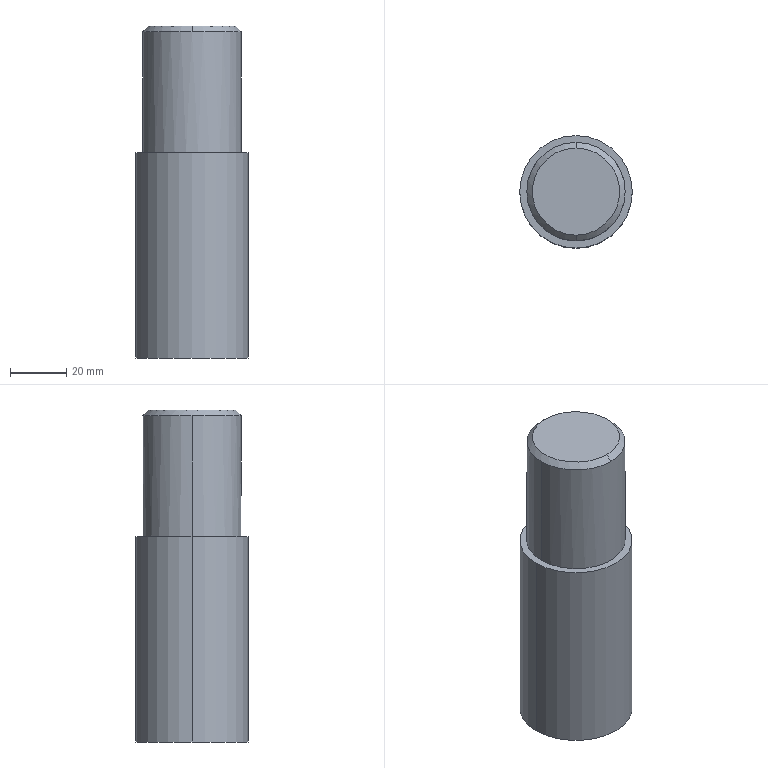Part | STEP file | PISTON XYLANH _S_^80 | 1 solid | 9 faces | box 40 x 40 x 118 mm | volume 134818 mm3 | cylinder 4 | plane 3 | cone 2 | commonest cylinder face diameters 35 x2 40 x2
STEP:
#1=CARTESIAN_POINT('',(0.,0.,0.));
#2=DIRECTION('',(0.,0.,1.));
#3=DIRECTION('',(1.,0.,0.));
#4=AXIS2_PLACEMENT_3D('',#1,#2,#3);
#5=CARTESIAN_POINT('',(20.,0.,0.));
#6=VERTEX_POINT('',#5);
#7=CARTESIAN_POINT('',(-20.,0.,0.));
#8=VERTEX_POINT('',#7);
#9=CARTESIAN_POINT('',(0.,0.,0.));
#10=DIRECTION('',(0.,0.,1.));
#11=DIRECTION('',(1.,0.,0.));
#12=AXIS2_PLACEMENT_3D('',#9,#10,#11);
#13=CIRCLE('',#12,20.);
#14=CARTESIAN_POINT('',(0.,0.,0.));
#15=DIRECTION('',(0.,0.,1.));
#16=DIRECTION('',(1.,0.,0.));
#17=AXIS2_PLACEMENT_3D('',#14,#15,#16);
#18=CYLINDRICAL_SURFACE('',#17,20.);
#19=CARTESIAN_POINT('',(0.,0.));
#20=DIRECTION('',(1.,0.));
#21=VECTOR('',#20,1.);
#22=LINE('',#19,#21);
#23=(GEOMETRIC_REPRESENTATION_CONTEXT(2)PARAMETRIC_REPRESENTATION_CONTEXT()REPRESENTATION_CONTEXT('',''));
#24=DEFINITIONAL_REPRESENTATION('',(#22),#23);
#25=PCURVE('',#18,#24);
#26=CARTESIAN_POINT('',(0.,0.,0.));
#27=DIRECTION('',(0.,0.,-1.));
#28=DIRECTION('',(-1.,0.,0.));
#29=AXIS2_PLACEMENT_3D('',#26,#27,#28);
#30=PLANE('',#29);
#31=CARTESIAN_POINT('',(-20.,0.));
#32=CARTESIAN_POINT('',(-20.,34.641));
#33=CARTESIAN_POINT('',(10.,17.321));
#34=CARTESIAN_POINT('',(40.,0.));
#35=CARTESIAN_POINT('',(10.,-17.321));
#36=CARTESIAN_POINT('',(-20.,-34.641));
#37=CARTESIAN_POINT('',(-20.,0.));
#38=(BOUNDED_CURVE()B_SPLINE_CURVE(2,(#31,#32,#33,#34,#35,#36,#37),.UNSPECIFIED.,.T.,.F.)B_SPLINE_CURVE_WITH_KNOTS((1,2,2,2,2,1),(-2.094,0.,2.094,4.189,6.283,8.378),.UNSPECIFIED.)CURVE()GEOMETRIC_REPRESENTATION_ITEM()RATIONAL_B_SPLINE_CURVE((1.,0.5,1.,0.5,1.,0.5,1.))REPRESENTATION_ITEM(''));
#39=(GEOMETRIC_REPRESENTATION_CONTEXT(2)PARAMETRIC_REPRESENTATION_CONTEXT()REPRESENTATION_CONTEXT('',''));
#40=DEFINITIONAL_REPRESENTATION('',(#38),#39);
#41=PCURVE('',#30,#40);
#42=SURFACE_CURVE('',#13,(#25,#41),.PCURVE_S1.);
#43=EDGE_CURVE('',#6,#8,#42,.T.);
#44=ORIENTED_EDGE('',*,*,#43,.T.);
#45=CARTESIAN_POINT('',(-20.,0.,73.));
#46=VERTEX_POINT('',#45);
#47=CARTESIAN_POINT('',(-20.,0.,0.));
#48=DIRECTION('',(0.,0.,1.));
#49=VECTOR('',#48,1.);
#50=LINE('',#47,#49);
#51=CARTESIAN_POINT('',(3.142,0.));
#52=DIRECTION('',(0.,1.));
#53=VECTOR('',#52,1.);
#54=LINE('',#51,#53);
#55=(GEOMETRIC_REPRESENTATION_CONTEXT(2)PARAMETRIC_REPRESENTATION_CONTEXT()REPRESENTATION_CONTEXT('',''));
#56=DEFINITIONAL_REPRESENTATION('',(#54),#55);
#57=PCURVE('',#18,#56);
#58=CARTESIAN_POINT('',(0.,0.,0.));
#59=DIRECTION('',(0.,0.,1.));
#60=DIRECTION('',(1.,0.,0.));
#61=AXIS2_PLACEMENT_3D('',#58,#59,#60);
#62=CYLINDRICAL_SURFACE('',#61,20.);
#63=CARTESIAN_POINT('',(3.142,0.));
#64=DIRECTION('',(0.,1.));
#65=VECTOR('',#64,1.);
#66=LINE('',#63,#65);
#67=(GEOMETRIC_REPRESENTATION_CONTEXT(2)PARAMETRIC_REPRESENTATION_CONTEXT()REPRESENTATION_CONTEXT('',''));
#68=DEFINITIONAL_REPRESENTATION('',(#66),#67);
#69=PCURVE('',#62,#68);
#70=SURFACE_CURVE('',#50,(#57,#69),.PCURVE_S1.);
#71=EDGE_CURVE('',#8,#46,#70,.T.);
#72=ORIENTED_EDGE('',*,*,#71,.T.);
#73=CARTESIAN_POINT('',(20.,0.,73.));
#74=VERTEX_POINT('',#73);
#75=CARTESIAN_POINT('',(0.,0.,73.));
#76=DIRECTION('',(0.,0.,-1.));
#77=DIRECTION('',(1.,0.,0.));
#78=AXIS2_PLACEMENT_3D('',#75,#76,#77);
#79=CIRCLE('',#78,20.);
#80=CARTESIAN_POINT('',(6.283,73.));
#81=DIRECTION('',(-1.,0.));
#82=VECTOR('',#81,1.);
#83=LINE('',#80,#82);
#84=(GEOMETRIC_REPRESENTATION_CONTEXT(2)PARAMETRIC_REPRESENTATION_CONTEXT()REPRESENTATION_CONTEXT('',''));
#85=DEFINITIONAL_REPRESENTATION('',(#83),#84);
#86=PCURVE('',#18,#85);
#87=CARTESIAN_POINT('',(0.,0.,73.));
#88=DIRECTION('',(0.,0.,-1.));
#89=DIRECTION('',(-1.,0.,0.));
#90=AXIS2_PLACEMENT_3D('',#87,#88,#89);
#91=PLANE('',#90);
#92=CARTESIAN_POINT('',(0.,0.));
#93=DIRECTION('',(-1.,0.));
#94=AXIS2_PLACEMENT_2D('',#92,#93);
#95=CIRCLE('',#94,20.);
#96=(GEOMETRIC_REPRESENTATION_CONTEXT(2)PARAMETRIC_REPRESENTATION_CONTEXT()REPRESENTATION_CONTEXT('',''));
#97=DEFINITIONAL_REPRESENTATION('',(#95),#96);
#98=PCURVE('',#91,#97);
#99=SURFACE_CURVE('',#79,(#86,#98),.PCURVE_S1.);
#100=EDGE_CURVE('',#46,#74,#99,.T.);
#101=ORIENTED_EDGE('',*,*,#100,.T.);
#102=CARTESIAN_POINT('',(20.,0.,0.));
#103=DIRECTION('',(0.,0.,1.));
#104=VECTOR('',#103,1.);
#105=LINE('',#102,#104);
#106=CARTESIAN_POINT('',(0.,0.));
#107=DIRECTION('',(0.,1.));
#108=VECTOR('',#107,1.);
#109=LINE('',#106,#108);
#110=(GEOMETRIC_REPRESENTATION_CONTEXT(2)PARAMETRIC_REPRESENTATION_CONTEXT()REPRESENTATION_CONTEXT('',''));
#111=DEFINITIONAL_REPRESENTATION('',(#109),#110);
#112=PCURVE('',#18,#111);
#113=CARTESIAN_POINT('',(6.283,0.));
#114=DIRECTION('',(0.,1.));
#115=VECTOR('',#114,1.);
#116=LINE('',#113,#115);
#117=(GEOMETRIC_REPRESENTATION_CONTEXT(2)PARAMETRIC_REPRESENTATION_CONTEXT()REPRESENTATION_CONTEXT('',''));
#118=DEFINITIONAL_REPRESENTATION('',(#116),#117);
#119=PCURVE('',#62,#118);
#120=SURFACE_CURVE('',#105,(#112,#119),.PCURVE_S1.);
#121=EDGE_CURVE('',#6,#74,#120,.T.);
#122=ORIENTED_EDGE('',*,*,#121,.F.);
#123=EDGE_LOOP('',(#44,#72,#101,#122));
#124=FACE_BOUND('',#123,.T.);
#125=ADVANCED_FACE('',(#124),#18,.T.);
#126=CARTESIAN_POINT('',(17.5,0.,73.));
#127=VERTEX_POINT('',#126);
#128=CARTESIAN_POINT('',(-17.5,0.,73.));
#129=VERTEX_POINT('',#128);
#130=CARTESIAN_POINT('',(0.,0.,73.));
#131=DIRECTION('',(0.,0.,1.));
#132=DIRECTION('',(1.,0.,0.));
#133=AXIS2_PLACEMENT_3D('',#130,#131,#132);
#134=CIRCLE('',#133,17.5);
#135=CARTESIAN_POINT('',(0.,0.,73.));
#136=DIRECTION('',(0.,0.,1.));
#137=DIRECTION('',(1.,0.,0.));
#138=AXIS2_PLACEMENT_3D('',#135,#136,#137);
#139=CYLINDRICAL_SURFACE('',#138,17.5);
#140=CARTESIAN_POINT('',(0.,0.));
#141=DIRECTION('',(1.,0.));
#142=VECTOR('',#141,1.);
#143=LINE('',#140,#142);
#144=(GEOMETRIC_REPRESENTATION_CONTEXT(2)PARAMETRIC_REPRESENTATION_CONTEXT()REPRESENTATION_CONTEXT('',''));
#145=DEFINITIONAL_REPRESENTATION('',(#143),#144);
#146=PCURVE('',#139,#145);
#147=CARTESIAN_POINT('',(-17.5,0.));
#148=CARTESIAN_POINT('',(-17.5,30.311));
#149=CARTESIAN_POINT('',(8.75,15.155));
#150=CARTESIAN_POINT('',(35.,0.));
#151=CARTESIAN_POINT('',(8.75,-15.155));
#152=CARTESIAN_POINT('',(-17.5,-30.311));
#153=CARTESIAN_POINT('',(-17.5,0.));
#154=(BOUNDED_CURVE()B_SPLINE_CURVE(2,(#147,#148,#149,#150,#151,#152,#153),.UNSPECIFIED.,.T.,.F.)B_SPLINE_CURVE_WITH_KNOTS((1,2,2,2,2,1),(-2.094,0.,2.094,4.189,6.283,8.378),.UNSPECIFIED.)CURVE()GEOMETRIC_REPRESENTATION_ITEM()RATIONAL_B_SPLINE_CURVE((1.,0.5,1.,0.5,1.,0.5,1.))REPRESENTATION_ITEM(''));
#155=(GEOMETRIC_REPRESENTATION_CONTEXT(2)PARAMETRIC_REPRESENTATION_CONTEXT()REPRESENTATION_CONTEXT('',''));
#156=DEFINITIONAL_REPRESENTATION('',(#154),#155);
#157=PCURVE('',#91,#156);
#158=SURFACE_CURVE('',#134,(#146,#157),.PCURVE_S1.);
#159=EDGE_CURVE('',#127,#129,#158,.T.);
#160=ORIENTED_EDGE('',*,*,#159,.T.);
#161=CARTESIAN_POINT('',(-17.5,0.,116.));
#162=VERTEX_POINT('',#161);
#163=CARTESIAN_POINT('',(-17.5,0.,73.));
#164=DIRECTION('',(0.,0.,1.));
#165=VECTOR('',#164,1.);
#166=LINE('',#163,#165);
#167=CARTESIAN_POINT('',(3.142,0.));
#168=DIRECTION('',(0.,1.));
#169=VECTOR('',#168,1.);
#170=LINE('',#167,#169);
#171=(GEOMETRIC_REPRESENTATION_CONTEXT(2)PARAMETRIC_REPRESENTATION_CONTEXT()REPRESENTATION_CONTEXT('',''));
#172=DEFINITIONAL_REPRESENTATION('',(#170),#171);
#173=PCURVE('',#139,#172);
#174=CARTESIAN_POINT('',(0.,0.,73.));
#175=DIRECTION('',(0.,0.,1.));
#176=DIRECTION('',(1.,0.,0.));
#177=AXIS2_PLACEMENT_3D('',#174,#175,#176);
#178=CYLINDRICAL_SURFACE('',#177,17.5);
#179=CARTESIAN_POINT('',(3.142,0.));
#180=DIRECTION('',(0.,1.));
#181=VECTOR('',#180,1.);
#182=LINE('',#179,#181);
#183=(GEOMETRIC_REPRESENTATION_CONTEXT(2)PARAMETRIC_REPRESENTATION_CONTEXT()REPRESENTATION_CONTEXT('',''));
#184=DEFINITIONAL_REPRESENTATION('',(#182),#183);
#185=PCURVE('',#178,#184);
#186=SURFACE_CURVE('',#166,(#173,#185),.PCURVE_S1.);
#187=EDGE_CURVE('',#129,#162,#186,.T.);
#188=ORIENTED_EDGE('',*,*,#187,.T.);
#189=CARTESIAN_POINT('',(0.,17.5,116.));
#190=VERTEX_POINT('',#189);
#191=CARTESIAN_POINT('',(0.,0.,116.));
#192=DIRECTION('',(0.,0.,-1.));
#193=DIRECTION('',(1.,0.,0.));
#194=AXIS2_PLACEMENT_3D('',#191,#192,#193);
#195=CIRCLE('',#194,17.5);
#196=CARTESIAN_POINT('',(6.283,43.));
#197=DIRECTION('',(-1.,0.));
#198=VECTOR('',#197,1.);
#199=LINE('',#196,#198);
#200=(GEOMETRIC_REPRESENTATION_CONTEXT(2)PARAMETRIC_REPRESENTATION_CONTEXT()REPRESENTATION_CONTEXT('',''));
#201=DEFINITIONAL_REPRESENTATION('',(#199),#200);
#202=PCURVE('',#139,#201);
#203=CARTESIAN_POINT('',(0.,0.,116.));
#204=DIRECTION('',(0.,0.,-1.));
#205=DIRECTION('',(0.,1.,0.));
#206=AXIS2_PLACEMENT_3D('',#203,#204,#205);
#207=CONICAL_SURFACE('',#206,17.5,0.7854);
#208=CARTESIAN_POINT('',(1.571,0.));
#209=DIRECTION('',(1.,0.));
#210=VECTOR('',#209,1.);
#211=LINE('',#208,#210);
#212=(GEOMETRIC_REPRESENTATION_CONTEXT(2)PARAMETRIC_REPRESENTATION_CONTEXT()REPRESENTATION_CONTEXT('',''));
#213=DEFINITIONAL_REPRESENTATION('',(#211),#212);
#214=PCURVE('',#207,#213);
#215=SURFACE_CURVE('',#195,(#202,#214),.PCURVE_S1.);
#216=EDGE_CURVE('',#162,#190,#215,.T.);
#217=ORIENTED_EDGE('',*,*,#216,.T.);
#218=CARTESIAN_POINT('',(17.5,0.,116.));
#219=VERTEX_POINT('',#218);
#220=CARTESIAN_POINT('',(0.,0.,116.));
#221=DIRECTION('',(0.,0.,-1.));
#222=DIRECTION('',(1.,0.,0.));
#223=AXIS2_PLACEMENT_3D('',#220,#221,#222);
#224=CIRCLE('',#223,17.5);
#225=CARTESIAN_POINT('',(6.283,43.));
#226=DIRECTION('',(-1.,0.));
#227=VECTOR('',#226,1.);
#228=LINE('',#225,#227);
#229=(GEOMETRIC_REPRESENTATION_CONTEXT(2)PARAMETRIC_REPRESENTATION_CONTEXT()REPRESENTATION_CONTEXT('',''));
#230=DEFINITIONAL_REPRESENTATION('',(#228),#229);
#231=PCURVE('',#139,#230);
#232=CARTESIAN_POINT('',(0.,0.,116.));
#233=DIRECTION('',(0.,0.,-1.));
#234=DIRECTION('',(0.,1.,0.));
#235=AXIS2_PLACEMENT_3D('',#232,#233,#234);
#236=CONICAL_SURFACE('',#235,17.5,0.7854);
#237=CARTESIAN_POINT('',(-4.712,0.));
#238=DIRECTION('',(1.,0.));
#239=VECTOR('',#238,1.);
#240=LINE('',#237,#239);
#241=(GEOMETRIC_REPRESENTATION_CONTEXT(2)PARAMETRIC_REPRESENTATION_CONTEXT()REPRESENTATION_CONTEXT('',''));
#242=DEFINITIONAL_REPRESENTATION('',(#240),#241);
#243=PCURVE('',#236,#242);
#244=SURFACE_CURVE('',#224,(#231,#243),.PCURVE_S1.);
#245=EDGE_CURVE('',#190,#219,#244,.T.);
#246=ORIENTED_EDGE('',*,*,#245,.T.);
#247=CARTESIAN_POINT('',(17.5,0.,73.));
#248=DIRECTION('',(0.,0.,1.));
#249=VECTOR('',#248,1.);
#250=LINE('',#247,#249);
#251=CARTESIAN_POINT('',(0.,0.));
#252=DIRECTION('',(0.,1.));
#253=VECTOR('',#252,1.);
#254=LINE('',#251,#253);
#255=(GEOMETRIC_REPRESENTATION_CONTEXT(2)PARAMETRIC_REPRESENTATION_CONTEXT()REPRESENTATION_CONTEXT('',''));
#256=DEFINITIONAL_REPRESENTATION('',(#254),#255);
#257=PCURVE('',#139,#256);
#258=CARTESIAN_POINT('',(6.283,0.));
#259=DIRECTION('',(0.,1.));
#260=VECTOR('',#259,1.);
#261=LINE('',#258,#260);
#262=(GEOMETRIC_REPRESENTATION_CONTEXT(2)PARAMETRIC_REPRESENTATION_CONTEXT()REPRESENTATION_CONTEXT('',''));
#263=DEFINITIONAL_REPRESENTATION('',(#261),#262);
#264=PCURVE('',#178,#263);
#265=SURFACE_CURVE('',#250,(#257,#264),.PCURVE_S1.);
#266=EDGE_CURVE('',#127,#219,#265,.T.);
#267=ORIENTED_EDGE('',*,*,#266,.F.);
#268=EDGE_LOOP('',(#160,#188,#217,#246,#267));
#269=FACE_BOUND('',#268,.T.);
#270=ADVANCED_FACE('',(#269),#139,.T.);
#271=CARTESIAN_POINT('',(0.,15.5,118.));
#272=VERTEX_POINT('',#271);
#273=CARTESIAN_POINT('',(0.,-15.5,118.));
#274=VERTEX_POINT('',#273);
#275=CARTESIAN_POINT('',(0.,0.,118.));
#276=DIRECTION('',(0.,0.,-1.));
#277=DIRECTION('',(0.,1.,0.));
#278=AXIS2_PLACEMENT_3D('',#275,#276,#277);
#279=CIRCLE('',#278,15.5);
#280=CARTESIAN_POINT('',(0.,-2.));
#281=DIRECTION('',(1.,0.));
#282=VECTOR('',#281,1.);
#283=LINE('',#280,#282);
#284=(GEOMETRIC_REPRESENTATION_CONTEXT(2)PARAMETRIC_REPRESENTATION_CONTEXT()REPRESENTATION_CONTEXT('',''));
#285=DEFINITIONAL_REPRESENTATION('',(#283),#284);
#286=PCURVE('',#236,#285);
#287=CARTESIAN_POINT('',(0.,0.,118.));
#288=DIRECTION('',(0.,0.,-1.));
#289=DIRECTION('',(-1.,0.,0.));
#290=AXIS2_PLACEMENT_3D('',#287,#288,#289);
#291=PLANE('',#290);
#292=CARTESIAN_POINT('',(0.,0.));
#293=DIRECTION('',(0.,1.));
#294=AXIS2_PLACEMENT_2D('',#292,#293);
#295=CIRCLE('',#294,15.5);
#296=(GEOMETRIC_REPRESENTATION_CONTEXT(2)PARAMETRIC_REPRESENTATION_CONTEXT()REPRESENTATION_CONTEXT('',''));
#297=DEFINITIONAL_REPRESENTATION('',(#295),#296);
#298=PCURVE('',#291,#297);
#299=SURFACE_CURVE('',#279,(#286,#298),.PCURVE_S1.);
#300=EDGE_CURVE('',#272,#274,#299,.T.);
#301=ORIENTED_EDGE('',*,*,#300,.T.);
#302=CARTESIAN_POINT('',(0.,-17.5,116.));
#303=VERTEX_POINT('',#302);
#304=CARTESIAN_POINT('',(0.,-17.5,116.));
#305=DIRECTION('',(0.,-0.7071,-0.7071));
#306=VECTOR('',#305,1.);
#307=LINE('',#304,#306);
#308=CARTESIAN_POINT('',(3.142,0.));
#309=DIRECTION('',(0.,1.));
#310=VECTOR('',#309,1.);
#311=LINE('',#308,#310);
#312=(GEOMETRIC_REPRESENTATION_CONTEXT(2)PARAMETRIC_REPRESENTATION_CONTEXT()REPRESENTATION_CONTEXT('',''));
#313=DEFINITIONAL_REPRESENTATION('',(#311),#312);
#314=PCURVE('',#236,#313);
#315=CARTESIAN_POINT('',(3.142,0.));
#316=DIRECTION('',(0.,1.));
#317=VECTOR('',#316,1.);
#318=LINE('',#315,#317);
#319=(GEOMETRIC_REPRESENTATION_CONTEXT(2)PARAMETRIC_REPRESENTATION_CONTEXT()REPRESENTATION_CONTEXT('',''));
#320=DEFINITIONAL_REPRESENTATION('',(#318),#319);
#321=PCURVE('',#207,#320);
#322=SURFACE_CURVE('',#307,(#314,#321),.PCURVE_S1.);
#323=EDGE_CURVE('',#274,#303,#322,.T.);
#324=ORIENTED_EDGE('',*,*,#323,.T.);
#325=CARTESIAN_POINT('',(0.,0.,116.));
#326=DIRECTION('',(0.,0.,-1.));
#327=DIRECTION('',(1.,0.,0.));
#328=AXIS2_PLACEMENT_3D('',#325,#326,#327);
#329=CIRCLE('',#328,17.5);
#330=CARTESIAN_POINT('',(1.571,0.));
#331=DIRECTION('',(1.,0.));
#332=VECTOR('',#331,1.);
#333=LINE('',#330,#332);
#334=(GEOMETRIC_REPRESENTATION_CONTEXT(2)PARAMETRIC_REPRESENTATION_CONTEXT()REPRESENTATION_CONTEXT('',''));
#335=DEFINITIONAL_REPRESENTATION('',(#333),#334);
#336=PCURVE('',#236,#335);
#337=CARTESIAN_POINT('',(6.283,43.));
#338=DIRECTION('',(-1.,0.));
#339=VECTOR('',#338,1.);
#340=LINE('',#337,#339);
#341=(GEOMETRIC_REPRESENTATION_CONTEXT(2)PARAMETRIC_REPRESENTATION_CONTEXT()REPRESENTATION_CONTEXT('',''));
#342=DEFINITIONAL_REPRESENTATION('',(#340),#341);
#343=PCURVE('',#178,#342);
#344=SURFACE_CURVE('',#329,(#336,#343),.PCURVE_S1.);
#345=EDGE_CURVE('',#219,#303,#344,.T.);
#346=ORIENTED_EDGE('',*,*,#345,.F.);
#347=ORIENTED_EDGE('',*,*,#245,.F.);
#348=CARTESIAN_POINT('',(0.,17.5,116.));
#349=DIRECTION('',(0.,0.7071,-0.7071));
#350=VECTOR('',#349,1.);
#351=LINE('',#348,#350);
#352=CARTESIAN_POINT('',(0.,0.));
#353=DIRECTION('',(0.,1.));
#354=VECTOR('',#353,1.);
#355=LINE('',#352,#354);
#356=(GEOMETRIC_REPRESENTATION_CONTEXT(2)PARAMETRIC_REPRESENTATION_CONTEXT()REPRESENTATION_CONTEXT('',''));
#357=DEFINITIONAL_REPRESENTATION('',(#355),#356);
#358=PCURVE('',#236,#357);
#359=CARTESIAN_POINT('',(6.283,0.));
#360=DIRECTION('',(0.,1.));
#361=VECTOR('',#360,1.);
#362=LINE('',#359,#361);
#363=(GEOMETRIC_REPRESENTATION_CONTEXT(2)PARAMETRIC_REPRESENTATION_CONTEXT()REPRESENTATION_CONTEXT('',''));
#364=DEFINITIONAL_REPRESENTATION('',(#362),#363);
#365=PCURVE('',#207,#364);
#366=SURFACE_CURVE('',#351,(#358,#365),.PCURVE_S1.);
#367=EDGE_CURVE('',#272,#190,#366,.T.);
#368=ORIENTED_EDGE('',*,*,#367,.F.);
#369=EDGE_LOOP('',(#301,#324,#346,#347,#368));
#370=FACE_BOUND('',#369,.T.);
#371=ADVANCED_FACE('',(#370),#236,.T.);
#372=ORIENTED_EDGE('',*,*,#71,.F.);
#373=CARTESIAN_POINT('',(0.,0.,0.));
#374=DIRECTION('',(0.,0.,1.));
#375=DIRECTION('',(1.,0.,0.));
#376=AXIS2_PLACEMENT_3D('',#373,#374,#375);
#377=CIRCLE('',#376,20.);
#378=CARTESIAN_POINT('',(0.,0.));
#379=DIRECTION('',(1.,0.));
#380=VECTOR('',#379,1.);
#381=LINE('',#378,#380);
#382=(GEOMETRIC_REPRESENTATION_CONTEXT(2)PARAMETRIC_REPRESENTATION_CONTEXT()REPRESENTATION_CONTEXT('',''));
#383=DEFINITIONAL_REPRESENTATION('',(#381),#382);
#384=PCURVE('',#62,#383);
#385=CARTESIAN_POINT('',(-20.,0.));
#386=CARTESIAN_POINT('',(-20.,34.641));
#387=CARTESIAN_POINT('',(10.,17.321));
#388=CARTESIAN_POINT('',(40.,0.));
#389=CARTESIAN_POINT('',(10.,-17.321));
#390=CARTESIAN_POINT('',(-20.,-34.641));
#391=CARTESIAN_POINT('',(-20.,0.));
#392=(BOUNDED_CURVE()B_SPLINE_CURVE(2,(#385,#386,#387,#388,#389,#390,#391),.UNSPECIFIED.,.T.,.F.)B_SPLINE_CURVE_WITH_KNOTS((1,2,2,2,2,1),(-2.094,0.,2.094,4.189,6.283,8.378),.UNSPECIFIED.)CURVE()GEOMETRIC_REPRESENTATION_ITEM()RATIONAL_B_SPLINE_CURVE((1.,0.5,1.,0.5,1.,0.5,1.))REPRESENTATION_ITEM(''));
#393=(GEOMETRIC_REPRESENTATION_CONTEXT(2)PARAMETRIC_REPRESENTATION_CONTEXT()REPRESENTATION_CONTEXT('',''));
#394=DEFINITIONAL_REPRESENTATION('',(#392),#393);
#395=PCURVE('',#30,#394);
#396=SURFACE_CURVE('',#377,(#384,#395),.PCURVE_S1.);
#397=EDGE_CURVE('',#8,#6,#396,.T.);
#398=ORIENTED_EDGE('',*,*,#397,.T.);
#399=ORIENTED_EDGE('',*,*,#121,.T.);
#400=CARTESIAN_POINT('',(0.,0.,73.));
#401=DIRECTION('',(0.,0.,-1.));
#402=DIRECTION('',(1.,0.,0.));
#403=AXIS2_PLACEMENT_3D('',#400,#401,#402);
#404=CIRCLE('',#403,20.);
#405=CARTESIAN_POINT('',(6.283,73.));
#406=DIRECTION('',(-1.,0.));
#407=VECTOR('',#406,1.);
#408=LINE('',#405,#407);
#409=(GEOMETRIC_REPRESENTATION_CONTEXT(2)PARAMETRIC_REPRESENTATION_CONTEXT()REPRESENTATION_CONTEXT('',''));
#410=DEFINITIONAL_REPRESENTATION('',(#408),#409);
#411=PCURVE('',#62,#410);
#412=CARTESIAN_POINT('',(0.,0.));
#413=DIRECTION('',(-1.,0.));
#414=AXIS2_PLACEMENT_2D('',#412,#413);
#415=CIRCLE('',#414,20.);
#416=(GEOMETRIC_REPRESENTATION_CONTEXT(2)PARAMETRIC_REPRESENTATION_CONTEXT()REPRESENTATION_CONTEXT('',''));
#417=DEFINITIONAL_REPRESENTATION('',(#415),#416);
#418=PCURVE('',#91,#417);
#419=SURFACE_CURVE('',#404,(#411,#418),.PCURVE_S1.);
#420=EDGE_CURVE('',#74,#46,#419,.T.);
#421=ORIENTED_EDGE('',*,*,#420,.T.);
#422=EDGE_LOOP('',(#372,#398,#399,#421));
#423=FACE_BOUND('',#422,.T.);
#424=ADVANCED_FACE('',(#423),#62,.T.);
#425=ORIENTED_EDGE('',*,*,#43,.F.);
#426=ORIENTED_EDGE('',*,*,#397,.F.);
#427=EDGE_LOOP('',(#425,#426));
#428=FACE_BOUND('',#427,.T.);
#429=ADVANCED_FACE('',(#428),#30,.T.);
#430=ORIENTED_EDGE('',*,*,#159,.F.);
#431=CARTESIAN_POINT('',(0.,0.,73.));
#432=DIRECTION('',(0.,0.,1.));
#433=DIRECTION('',(1.,0.,0.));
#434=AXIS2_PLACEMENT_3D('',#431,#432,#433);
#435=CIRCLE('',#434,17.5);
#436=CARTESIAN_POINT('',(-17.5,0.));
#437=CARTESIAN_POINT('',(-17.5,30.311));
#438=CARTESIAN_POINT('',(8.75,15.155));
#439=CARTESIAN_POINT('',(35.,0.));
#440=CARTESIAN_POINT('',(8.75,-15.155));
#441=CARTESIAN_POINT('',(-17.5,-30.311));
#442=CARTESIAN_POINT('',(-17.5,0.));
#443=(BOUNDED_CURVE()B_SPLINE_CURVE(2,(#436,#437,#438,#439,#440,#441,#442),.UNSPECIFIED.,.T.,.F.)B_SPLINE_CURVE_WITH_KNOTS((1,2,2,2,2,1),(-2.094,0.,2.094,4.189,6.283,8.378),.UNSPECIFIED.)CURVE()GEOMETRIC_REPRESENTATION_ITEM()RATIONAL_B_SPLINE_CURVE((1.,0.5,1.,0.5,1.,0.5,1.))REPRESENTATION_ITEM(''));
#444=(GEOMETRIC_REPRESENTATION_CONTEXT(2)PARAMETRIC_REPRESENTATION_CONTEXT()REPRESENTATION_CONTEXT('',''));
#445=DEFINITIONAL_REPRESENTATION('',(#443),#444);
#446=PCURVE('',#91,#445);
#447=CARTESIAN_POINT('',(0.,0.));
#448=DIRECTION('',(1.,0.));
#449=VECTOR('',#448,1.);
#450=LINE('',#447,#449);
#451=(GEOMETRIC_REPRESENTATION_CONTEXT(2)PARAMETRIC_REPRESENTATION_CONTEXT()REPRESENTATION_CONTEXT('',''));
#452=DEFINITIONAL_REPRESENTATION('',(#450),#451);
#453=PCURVE('',#178,#452);
#454=SURFACE_CURVE('',#435,(#446,#453),.PCURVE_S1.);
#455=EDGE_CURVE('',#129,#127,#454,.T.);
#456=ORIENTED_EDGE('',*,*,#455,.F.);
#457=EDGE_LOOP('',(#430,#456));
#458=FACE_BOUND('',#457,.T.);
#459=ORIENTED_EDGE('',*,*,#420,.F.);
#460=ORIENTED_EDGE('',*,*,#100,.F.);
#461=EDGE_LOOP('',(#459,#460));
#462=FACE_BOUND('',#461,.T.);
#463=ADVANCED_FACE('',(#458,#462),#91,.F.);
#464=ORIENTED_EDGE('',*,*,#187,.F.);
#465=ORIENTED_EDGE('',*,*,#455,.T.);
#466=ORIENTED_EDGE('',*,*,#266,.T.);
#467=ORIENTED_EDGE('',*,*,#345,.T.);
#468=CARTESIAN_POINT('',(0.,0.,116.));
#469=DIRECTION('',(0.,0.,-1.));
#470=DIRECTION('',(1.,0.,0.));
#471=AXIS2_PLACEMENT_3D('',#468,#469,#470);
#472=CIRCLE('',#471,17.5);
#473=CARTESIAN_POINT('',(6.283,43.));
#474=DIRECTION('',(-1.,0.));
#475=VECTOR('',#474,1.);
#476=LINE('',#473,#475);
#477=(GEOMETRIC_REPRESENTATION_CONTEXT(2)PARAMETRIC_REPRESENTATION_CONTEXT()REPRESENTATION_CONTEXT('',''));
#478=DEFINITIONAL_REPRESENTATION('',(#476),#477);
#479=PCURVE('',#178,#478);
#480=CARTESIAN_POINT('',(1.571,0.));
#481=DIRECTION('',(1.,0.));
#482=VECTOR('',#481,1.);
#483=LINE('',#480,#482);
#484=(GEOMETRIC_REPRESENTATION_CONTEXT(2)PARAMETRIC_REPRESENTATION_CONTEXT()REPRESENTATION_CONTEXT('',''));
#485=DEFINITIONAL_REPRESENTATION('',(#483),#484);
#486=PCURVE('',#207,#485);
#487=SURFACE_CURVE('',#472,(#479,#486),.PCURVE_S1.);
#488=EDGE_CURVE('',#303,#162,#487,.T.);
#489=ORIENTED_EDGE('',*,*,#488,.T.);
#490=EDGE_LOOP('',(#464,#465,#466,#467,#489));
#491=FACE_BOUND('',#490,.T.);
#492=ADVANCED_FACE('',(#491),#178,.T.);
#493=ORIENTED_EDGE('',*,*,#323,.F.);
#494=CARTESIAN_POINT('',(0.,0.,118.));
#495=DIRECTION('',(0.,0.,-1.));
#496=DIRECTION('',(0.,1.,0.));
#497=AXIS2_PLACEMENT_3D('',#494,#495,#496);
#498=CIRCLE('',#497,15.5);
#499=CARTESIAN_POINT('',(0.,-2.));
#500=DIRECTION('',(1.,0.));
#501=VECTOR('',#500,1.);
#502=LINE('',#499,#501);
#503=(GEOMETRIC_REPRESENTATION_CONTEXT(2)PARAMETRIC_REPRESENTATION_CONTEXT()REPRESENTATION_CONTEXT('',''));
#504=DEFINITIONAL_REPRESENTATION('',(#502),#503);
#505=PCURVE('',#207,#504);
#506=CARTESIAN_POINT('',(0.,0.));
#507=DIRECTION('',(0.,1.));
#508=AXIS2_PLACEMENT_2D('',#506,#507);
#509=CIRCLE('',#508,15.5);
#510=(GEOMETRIC_REPRESENTATION_CONTEXT(2)PARAMETRIC_REPRESENTATION_CONTEXT()REPRESENTATION_CONTEXT('',''));
#511=DEFINITIONAL_REPRESENTATION('',(#509),#510);
#512=PCURVE('',#291,#511);
#513=SURFACE_CURVE('',#498,(#505,#512),.PCURVE_S1.);
#514=EDGE_CURVE('',#274,#272,#513,.T.);
#515=ORIENTED_EDGE('',*,*,#514,.T.);
#516=ORIENTED_EDGE('',*,*,#367,.T.);
#517=ORIENTED_EDGE('',*,*,#216,.F.);
#518=ORIENTED_EDGE('',*,*,#488,.F.);
#519=EDGE_LOOP('',(#493,#515,#516,#517,#518));
#520=FACE_BOUND('',#519,.T.);
#521=ADVANCED_FACE('',(#520),#207,.T.);
#522=ORIENTED_EDGE('',*,*,#300,.F.);
#523=ORIENTED_EDGE('',*,*,#514,.F.);
#524=EDGE_LOOP('',(#522,#523));
#525=FACE_BOUND('',#524,.T.);
#526=ADVANCED_FACE('',(#525),#291,.F.);
#527=CLOSED_SHELL('',(#125,#270,#371,#424,#429,#463,#492,#521,#526));
#528=MANIFOLD_SOLID_BREP('',#527);
#529=(LENGTH_UNIT()NAMED_UNIT(*)SI_UNIT(.MILLI.,.METRE.));
#530=UNCERTAINTY_MEASURE_WITH_UNIT(LENGTH_MEASURE(0.0000001),#529,'','');
#531=(NAMED_UNIT(*)PLANE_ANGLE_UNIT()SI_UNIT($,.RADIAN.));
#532=(NAMED_UNIT(*)SI_UNIT($,.STERADIAN.)SOLID_ANGLE_UNIT());
#533=(GEOMETRIC_REPRESENTATION_CONTEXT(3)GLOBAL_UNCERTAINTY_ASSIGNED_CONTEXT((#530))GLOBAL_UNIT_ASSIGNED_CONTEXT((#529,#531,#532))REPRESENTATION_CONTEXT('',''));
#534=ADVANCED_BREP_SHAPE_REPRESENTATION('',(#4,#528),#533);